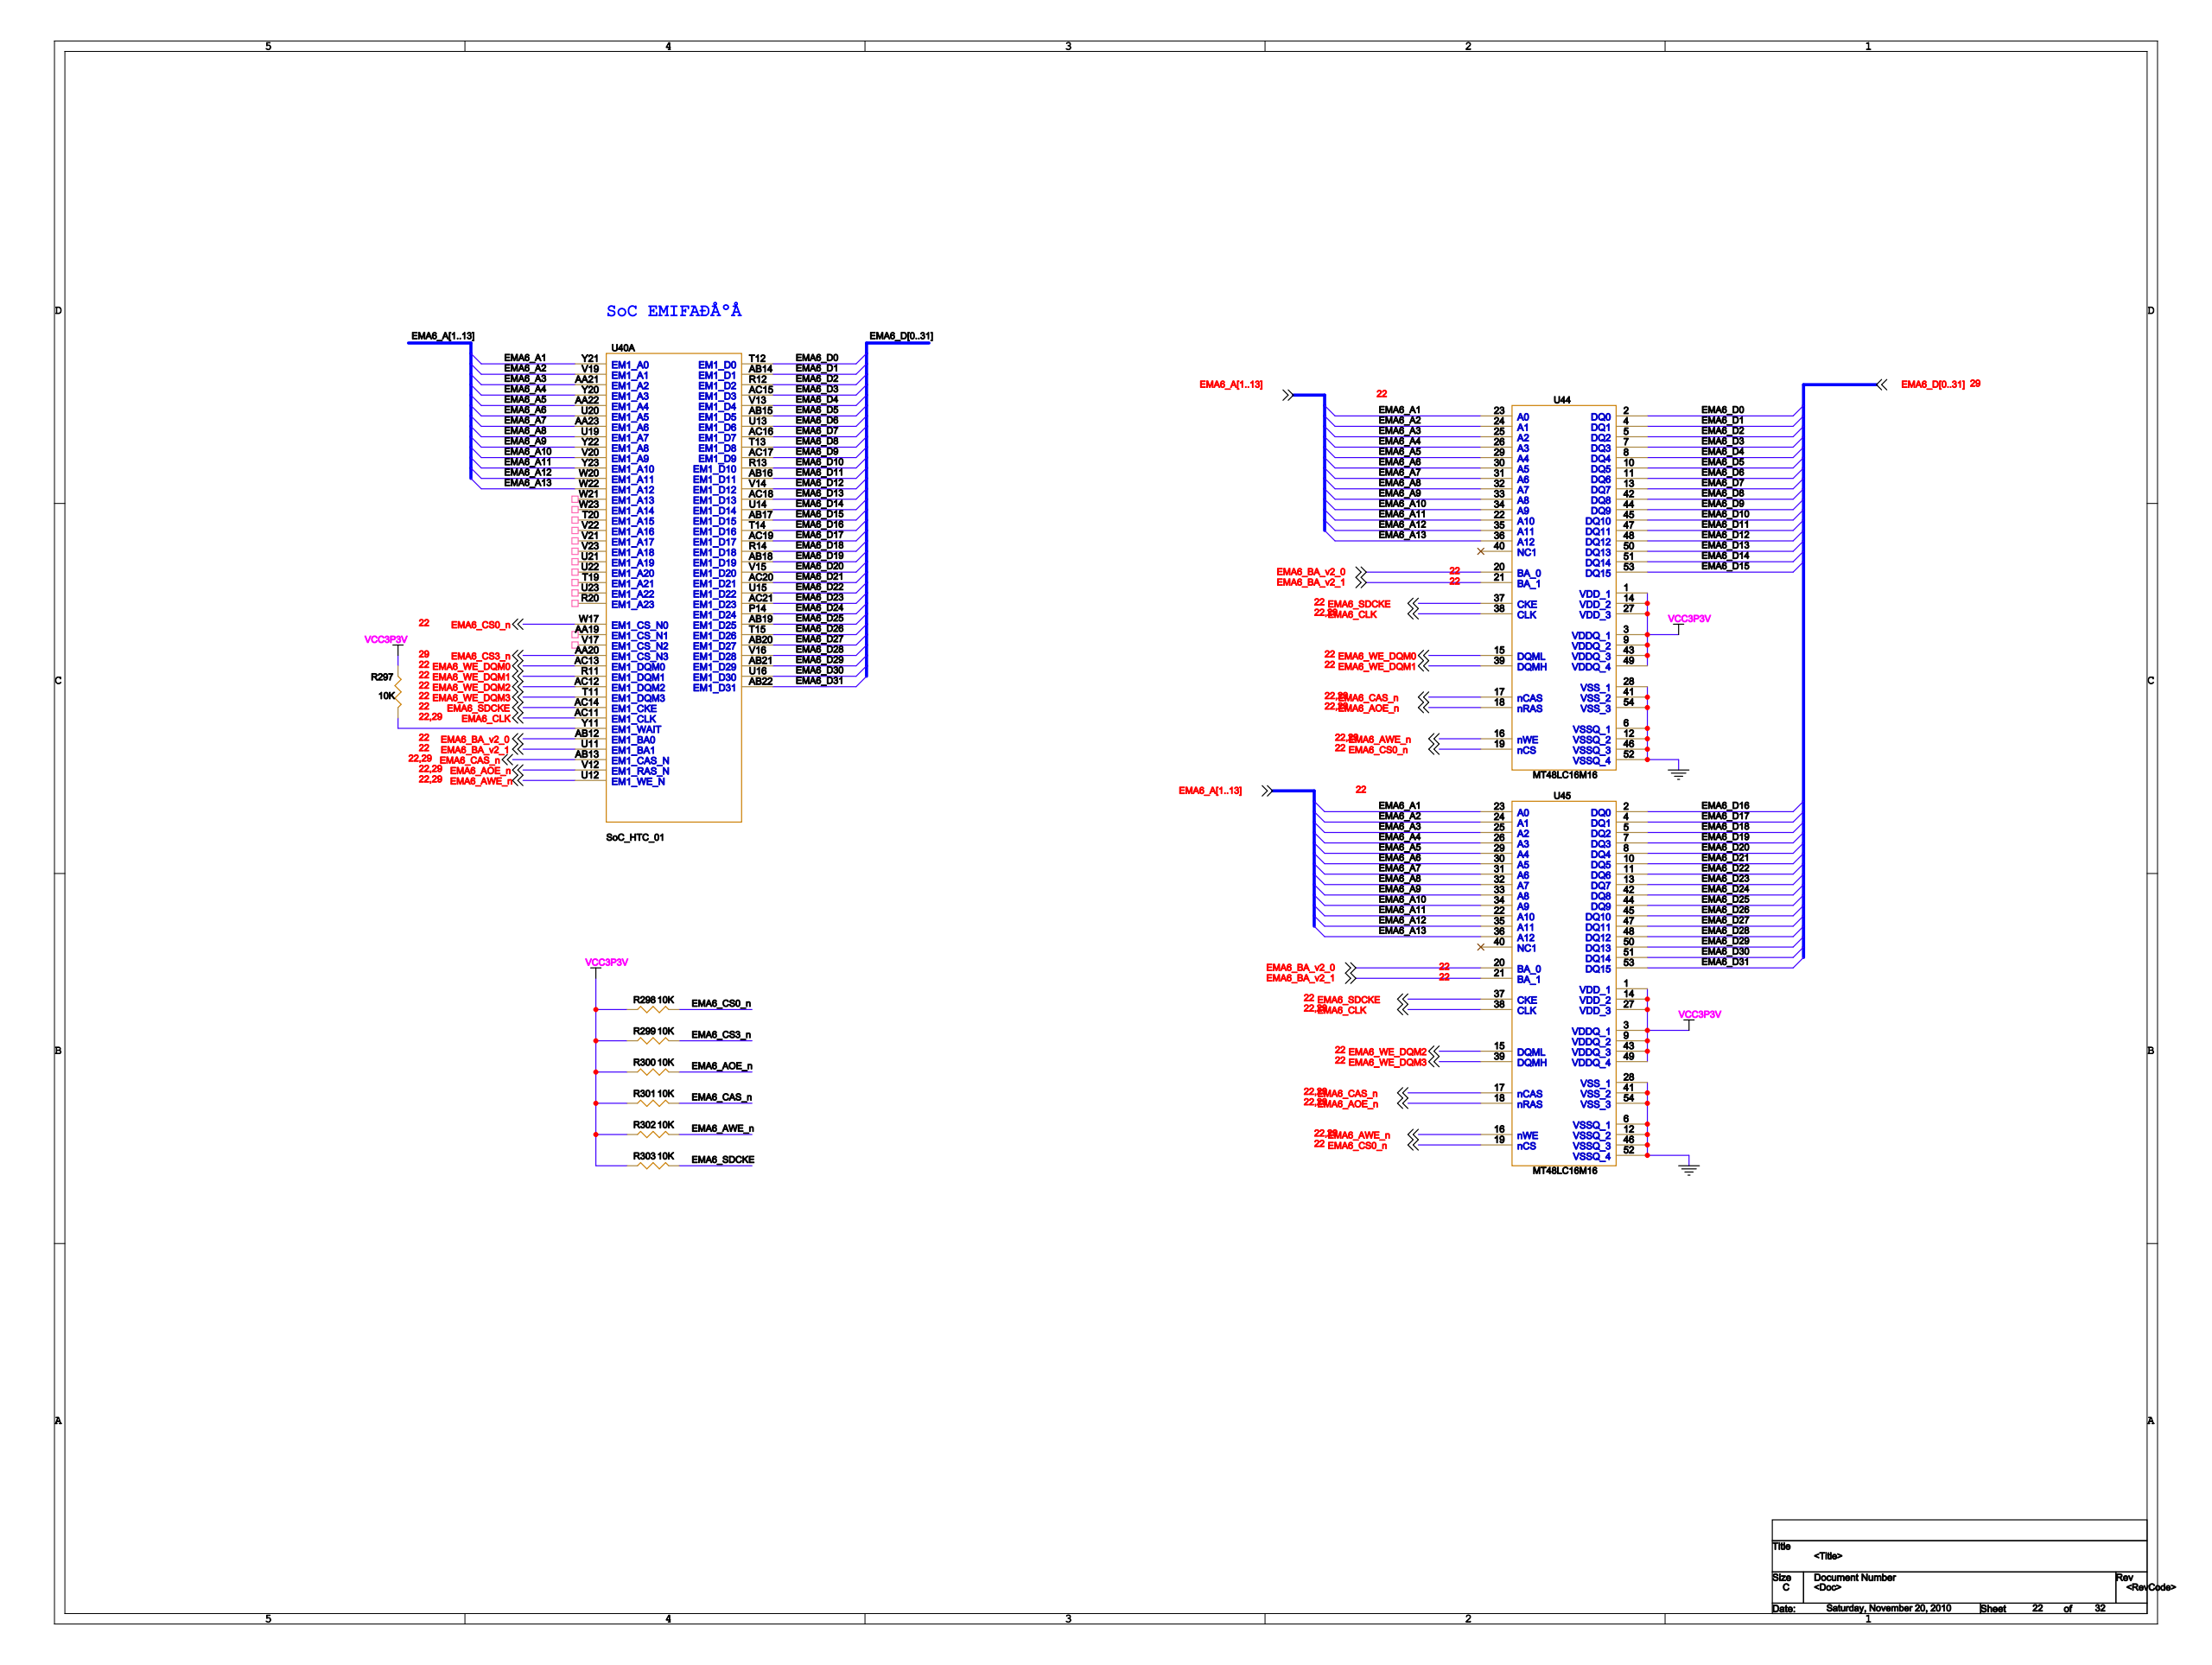Circuit board | Cadence Allegro | 1001 parts | 1318 nets | one sheet of the schematic
Parts on this sheet (reference | value | footprint):
R297 | 10K | 0603
R298 | 10K | 0603
R299 | 10K | 0603
R300 | 10K | 0603
R301 | 10K | 0603
R302 | 10K | 0603
R303 | 10K | 0603
U11 | MT48LC32M16 | TSOP54
U14 | MT48LC16M16 | TSOP54
U15 | MT48LC16M16 | TSOP54
U20 | MT48LC16M16 | TSOP54
U21 | MT48LC16M16 | TSOP54
U23 | MT48LC32M16 | TSOP54
U40 | SoC_HTC_01 | L529_XIN
U44 | MT48LC16M16 | TSOP54
U45 | MT48LC16M16 | TSOP54
Nets of these parts (net: part-pin ...):
EMA6_D13: U40-AC18 U44-50
EMA6_D19: U40-AB18 U45-7
EMA6_D25: U40-AB19 U45-44
EMA6_D28: U40-V16 U45-48
EMA6_D30: U40-U16 U45-51
EMA6_CS3_N: R299-2 U40-AA20
EMA6_D20: U40-V15 U45-8
EMA6_D31: U40-AB22 U45-53
EMA6_D27: U40-AB20 U45-47
EMA6_D17: U40-AC19 U45-4
EMA6_D21: U40-AC20 U45-10
EMA6_D29: U40-AB21 U45-50
EMA6_D23: U40-AC21 U45-13
EMA6_D26: U40-T15 U45-45
EMA6_D14: U40-U14 U44-51
EMA6_D22: U40-U15 U45-11
EMA6_D12: U40-V14 U44-48
EMA6_D5: U40-AB15 U44-10
EMA6_D3: U40-AC15 U44-7
EMA6_D9: U40-AC17 U44-44
EMA6_D15: U40-AB17 U44-53
EMA6_CAS_N: R301-2 U40-AB13 U44-17 U45-17
EMA6_D1: U40-AB14 U44-4
EMA6_D16: U40-T14 U45-2
EMA6_D11: U40-AB16 U44-47
EMA6_D0: U40-T12 U44-2
EMA6_D7: U40-AC16 U44-13
EMA6_D18: U40-R14 U45-5
EMA6_D8: U40-T13 U44-42
EMA6_D6: U40-U13 U44-11
EMA6_D2: U40-R12 U44-5
EMA6_D10: U40-R13 U44-45
EMA6_D24: U40-P14 U45-42
EMA6_AOE_N: R300-2 U40-V12 U44-18 U45-18
EMA6_D4: U40-V13 U44-8
EMA6_AWE_N: R302-2 U40-U12 U44-16 U45-16
EMA6_CLK: U40-AC11 U44-38 U45-38
VCC3P3V: R297-2 R298-1 R299-1 R300-1 R301-1 R302-1 R303-1 U11-1 U11-3 U11-9 U11-14 U11-27 U11-43 U11-49 U14-1 U14-3 U14-9 U14-14 U14-27 U14-43 U14-49 U15-1 U15-3 U15-9 U15-14 U15-27 U15-43 U15-49 U20-1 U20-3 U20-9 U20-14 U20-27 U20-43 U20-49 U21-1 U21-3 U21-9 U21-14 U21-27 U21-43 U21-49 U23-1 U23-3 U23-9 U23-14 U23-27 U23-43 U23-49 U44-1 U44-3 U44-9 U44-14 U44-27 U44-43 U44-49 U45-1 U45-3 U45-9 U45-14 U45-27 U45-43 U45-49
EMA6_A1: U40-Y21 U44-23 U45-23
EMA6_A2: U40-V19 U44-24 U45-24
EMA6_A11: U40-Y23 U44-22 U45-22
EMA6_A12: U40-W20 U44-35 U45-35
EMA6_A13: U40-W22 U44-36 U45-36
EMA6_A3: U40-AA21 U44-25 U45-25
EMA6_A4: U40-Y20 U44-26 U45-26
EMA6_A5: U40-AA22 U44-29 U45-29
EMA6_A6: U40-U20 U44-30 U45-30
EMA6_A7: U40-AA23 U44-31 U45-31
EMA6_A8: U40-U19 U44-32 U45-32
EMA6_A9: U40-Y22 U44-33 U45-33
EMA6_A10: U40-V20 U44-34 U45-34
EMA6_SDCKE: R303-2 U40-AC14 U44-37 U45-37
EMA6_CS0_N: R298-2 U40-W17 U44-19 U45-19
EMA6_WE_DQM0: U40-AC13 U44-15
EMA6_WE_DQM1: U40-R11 U44-39
EMA6_WE_DQM2: U40-AC12 U45-15
EMA6_WE_DQM3: U40-T11 U45-39
N16920859: R297-1 U40-Y11